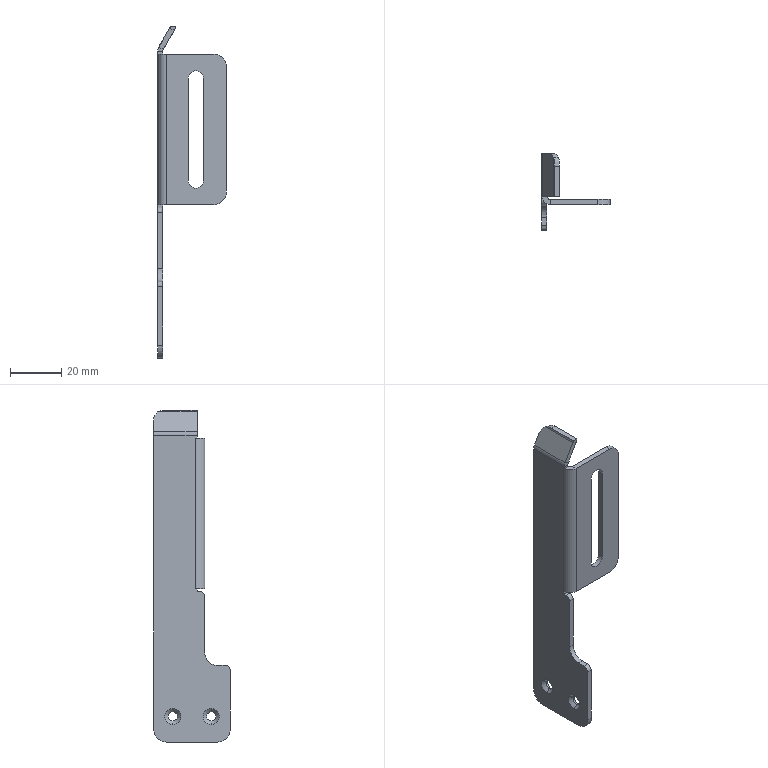Part | STEP file | BPSP-11-008Guide Plate_Default | 1 solid | 54 faces | box 27 x 30 x 130 mm | volume 7946 mm3 | plane 29 | cylinder 20 | cone 4 | spline 1 | commonest cylinder face diameters 10 x6 3.6 x4 3 x3 7 x3 4 x2 6 x2